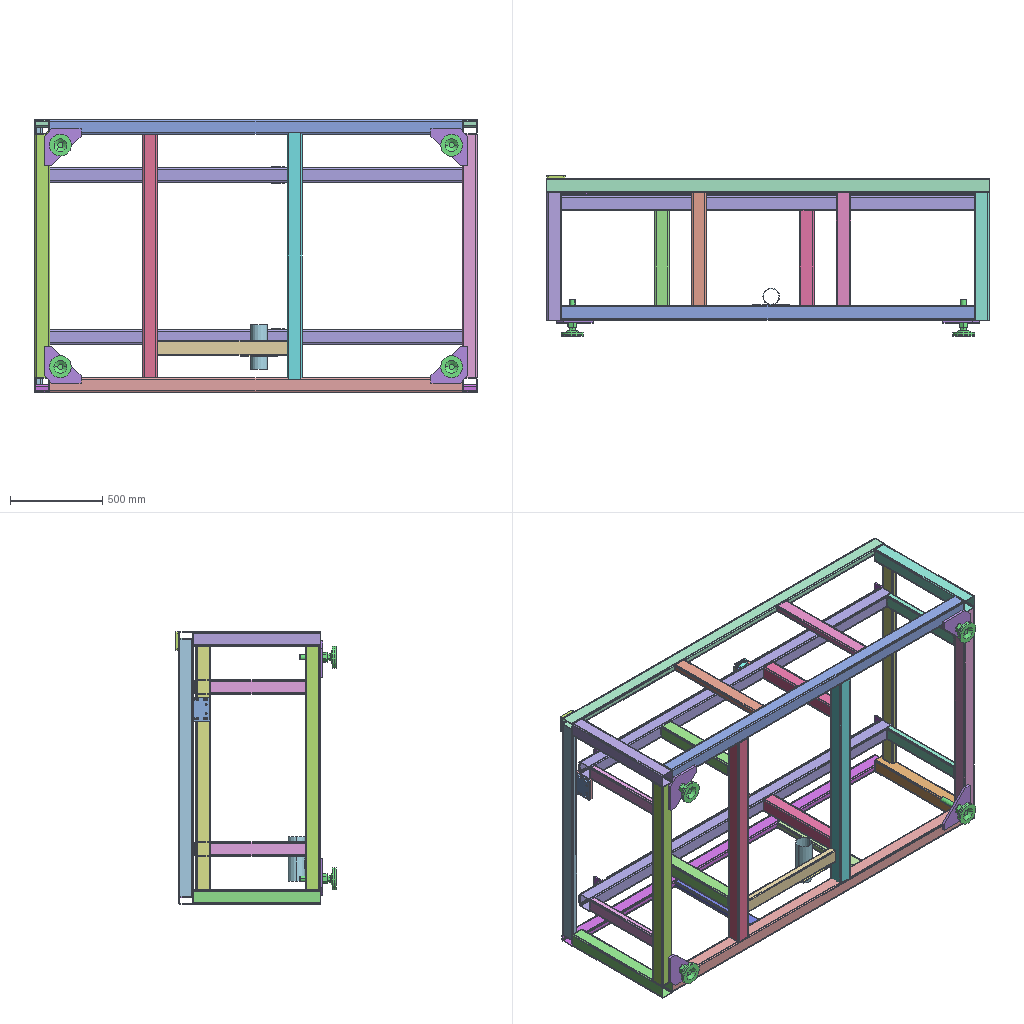Assembly | SolidWorks | 12 different items | 25 placed | box 2400 x 871 x 1480 mm
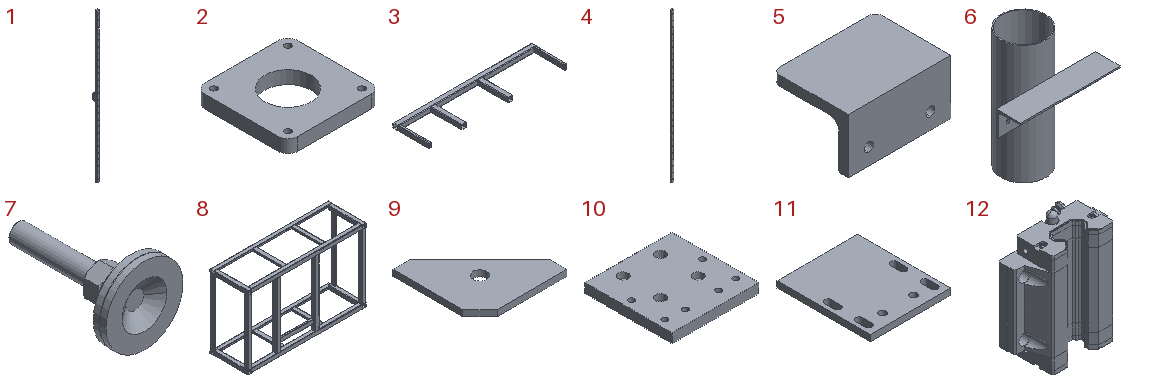Parts list (item | name | quantity | parent item | size | volume | features):
1 | (subassembly) | x2 | - | 90 x 42.01 x 2080 mm | 1460108 mm3 | features LocalLPattern 1
2 | - | x1 | - | 100 x 100 x 14 mm | 109276 mm3 | features ICE 2, Extrusion 1, Fillet 1, HoleWzd 1
3 | - | x2 | - | 2320 x 602 x 80 mm | 5618021 mm3 | features WeldMemberFeat 3, ICE 2, WeldCornerFeat 2, HoleWzd 1, LPattern 1, WeldmentFeature 1
4 | - | x2 | in 1 | 28 x 26 x 2080 mm | 1265174 mm3 | features ICE 19, MirrorPattern 5, Extrusion 4, MirrorSolid 4, Chamfer 3, Fillet 3, RevCut 3, Dome 2, LPattern 2, DeleteBody 1, LibraryFeature 1, Revolution 1
5 | - | x4 | - | 75 x 55 x 40 mm | 46347 mm3 | features 3DProfileFeature 1, Fillet 1, HoleWzd 1, ICE 1, WeldMemberFeat 1, WeldmentFeature 1
6 | - | x1 | - | 200 x 140 x 240 mm | 210373 mm3 | features 3DProfileFeature 1, HoleWzd 1, ICE 1, WeldMemberFeat 1, WeldmentFeature 1
7 | - | x4 | - | 120 x 197 x 120 mm | 378664 mm3 | features ICE 2, RevCut 2, Chamfer 1, Revolution 1
8 | - | x1 | - | 2400 x 770 x 1480 mm | 23706901 mm3 | features WeldCornerFeat 5, WeldMemberFeat 4, 3DProfileFeature 2, WeldmentFeature 1
9 | - | x4 | - | 200 x 200 x 14 mm | 358341 mm3 | features Extrusion 1
10 | - | x1 | - | 130 x 130 x 14 mm | 224199 mm3 | features HoleWzd 3, Extrusion 1, ICE 1
11 | - | x1 | - | 130 x 150 x 10 mm | 182698 mm3 | features HoleWzd 2, ICE 2, Extrusion 1
12 | - | x2 | in 1 | 90 x 36.51 x 110.4 mm | 194935 mm3 | features ICE 23, Extrusion 5, MirrorPattern 5, Fillet 4, MirrorSolid 4, Chamfer 3, RevCut 3, Dome 2, LPattern 2, Revolution 2, DeleteBody 1, LibraryFeature 1
Mates (type | each side: item.copy, entity, surface, feature):
In the top assembly
Coincident | 8.1 face plane Gb/6728-1986 Square Hollow Section 080 X 80 X 4(1) | 9.1 face plane Boss-Extrude1
DistanceDim | 9.1 face plane Boss-Extrude1 | 8.1 face plane Gb/6728-1986 Square Hollow Section 080 X 80 X 4(1) | 2 times
Coincident | 8.1 face plane Gb/6728-1986 Square Hollow Section 080 X 80 X 4(1) | 9.2 face plane Boss-Extrude1
DistanceDim | 9.2 face plane Boss-Extrude1 | 8.1 face plane Gb/6728-1986 Square Hollow Section 080 X 80 X 4(1) | 2 times
Coincident | 8.1 face plane Gb/6728-1986 Square Hollow Section 080 X 80 X 4(1) | 9.3 face plane Boss-Extrude1
DistanceDim | 8.1 face plane Gb/6728-1986 Square Hollow Section 080 X 80 X 4(1) | 9.3 face plane Boss-Extrude1
DistanceDim | 9.3 face plane Boss-Extrude1 | 8.1 face plane Gb/6728-1986 Square Hollow Section 080 X 80 X 4(1)
Coincident | 8.1 face plane Gb/6728-1986 Square Hollow Section 080 X 80 X 4(1) | 9.4 face plane Boss-Extrude1
DistanceDim | 9.4 face plane Boss-Extrude1 | 8.1 face plane Gb/6728-1986 Square Hollow Section 080 X 80 X 4(1)
DistanceDim | 8.1 face plane Gb/6728-1986 Square Hollow Section 080 X 80 X 4(1) | 9.4 face plane Boss-Extrude1
Concentric | 7.1 face cylinder Revolve1 | 9.2 face cylinder Boss-Extrude1
Coincident | 7.1 face plane Boss-Extrude2 | 9.2 face plane Boss-Extrude1
Coincident | 9.3 face plane Boss-Extrude1 | 7.2 face plane Boss-Extrude2
Concentric | 9.3 face cylinder Boss-Extrude1 | 7.2 face cylinder Revolve1
Coincident | 9.4 face plane Boss-Extrude1 | 7.3 face plane Boss-Extrude2
Concentric | 9.4 face cylinder Boss-Extrude1 | 7.3 face cylinder Revolve1
Coincident | 9.1 face plane Boss-Extrude1 | 7.4 face plane Boss-Extrude2
Concentric | 9.1 face cylinder Boss-Extrude1 | 7.4 face cylinder Revolve1
Coincident | 10.1 face plane Boss-Extrude1 | 11.1 face plane Boss-Extrude1
Concentric | 10.1 face cylinder M10 Tapped Hole1 | 11.1 face cylinder Ø11.0 (11) Diameter Hole1 | 2 times
Coincident | assembly face | assembly face | 2 times
Coincident | 8.1 face plane Gb/6728-1986 Square Hollow Section 080 X 80 X 4(1) | 3.1 face plane Gb/6728-1986 Rectangular Hollow Section 080 X 40 X 4(1)
Coincident | 8.1 face plane Gb/6728-1986 Rectangular Hollow Section 080 X 40 X 4(1) | 3.1 face plane Gb/6728-1986 Rectangular Hollow Section 080 X 40 X 4(1)
Coincident | 3.1 face plane Gb/6728-1986 Square Hollow Section 080 X 80 X 4(1) | 3.2 face plane Gb/6728-1986 Square Hollow Section 080 X 80 X 4(1)
Coincident | 3.1 face plane Gb/6728-1986 Rectangular Hollow Section 080 X 40 X 4(1) | 3.2 face plane Gb/6728-1986 Rectangular Hollow Section 080 X 40 X 4(1)
DistanceDim | 3.1 face plane Gb/6728-1986 Square Hollow Section 080 X 80 X 4(1) | 3.2 face plane Gb/6728-1986 Square Hollow Section 080 X 80 X 4(1)
Width | 8.1 face plane Gb/6728-1986 Rectangular Hollow Section 080 X 40 X 4(1) | 8.1 face plane Gb/6728-1986 Rectangular Hollow Section 080 X 40 X 4(1) | 3.1 face plane Gb/6728-1986 Square Hollow Section 080 X 80 X 4(1) | 3.2 face plane Gb/6728-1986 Square Hollow Section 080 X 80 X 4(1)
Coincident | assembly face | 3.2 face plane Gb/6728-1986 Square Hollow Section 080 X 80 X 4(1)
Width | 3.2 face plane Gb/6728-1986 Square Hollow Section 080 X 80 X 4(1) | 3.2 face plane Gb/6728-1986 Square Hollow Section 080 X 80 X 4(1) | assembly face
Coincident | 8.1 face plane Gb/6728-1986 Rectangular Hollow Section 080 X 40 X 4(1) | 2.1 face plane Boss-Extrude1 | 3 times
Coincident | 8.1 face plane Gb/6728-1986 Rectangular Hollow Section 080 X 40 X 4(1) | 11.1 face plane Boss-Extrude1
DistanceDim | 11.1 face plane Boss-Extrude2 | 8.1 face plane Gb/6728-1986 Rectangular Hollow Section 080 X 40 X 4(1)
DistanceDim | 10.1 face plane Boss-Extrude1 | 8.1 face plane Gb/6728-1986 Rectangular Hollow Section 080 X 40 X 4(1)
Coincident | 8.1 face plane Gb/6728-1986 Rectangular Hollow Section 080 X 40 X 3(1) | 6.1 face plane Equal Angle Steel 5X4(1) | 2 times
Width | 8.1 face plane Gb/6728-1986 Rectangular Hollow Section 080 X 40 X 4(1) | 8.1 face plane Gb/6728-1986 Rectangular Hollow Section 080 X 40 X 4(1) | 6.1 face cylinder Boss-Extrude1
Coincident | 8.1 face plane Gb/6728-1986 Rectangular Hollow Section 080 X 40 X 4(1) | 5.1 face plane Unequal Angle Steel 6.3-4(1)
Width | 5.1 face plane Unequal Angle Steel 6.3-4(1) | 5.1 face plane Unequal Angle Steel 6.3-4(1) | 3.2 face plane Gb/6728-1986 Square Hollow Section 080 X 80 X 4(1) | 3.2 face plane Gb/6728-1986 Square Hollow Section 080 X 80 X 4(1)
Coincident | 3.2 face plane Cut-Extrude1 | 5.2 face plane Unequal Angle Steel 6.3-4(1)
Coincident | 5.1 face plane Unequal Angle Steel 6.3-4(1) | 5.2 face plane Unequal Angle Steel 6.3-4(1)
Coincident | 3.2 face plane Cut-Extrude1 | 4.1 face plane Boss-Extrude10
Concentric | 3.2 face cylinder M8 Tapped Hole1 | 4.1 face cylinder Cut-Revolve2
Parallel | 3.2 face plane Gb/6728-1986 Square Hollow Section 080 X 80 X 4(1) | 4.1 face plane Boss-Extrude10
Coincident | 3.1 face plane Cut-Extrude1 | 4.2 face plane Boss-Extrude10
Concentric | 3.1 face cylinder M8 Tapped Hole1 | 4.2 face cylinder Cut-Revolve2
Parallel | 3.1 face plane Gb/6728-1986 Square Hollow Section 080 X 80 X 4(1) | 4.2 face plane Boss-Extrude10
In subassembly 1
Coincident | 12.1 face plane Cut-Extrude11 | 4.3 face plane Boss-Extrude10 | 2 times
Path | 12.1 select_type:25 | 4.3 select_type:0